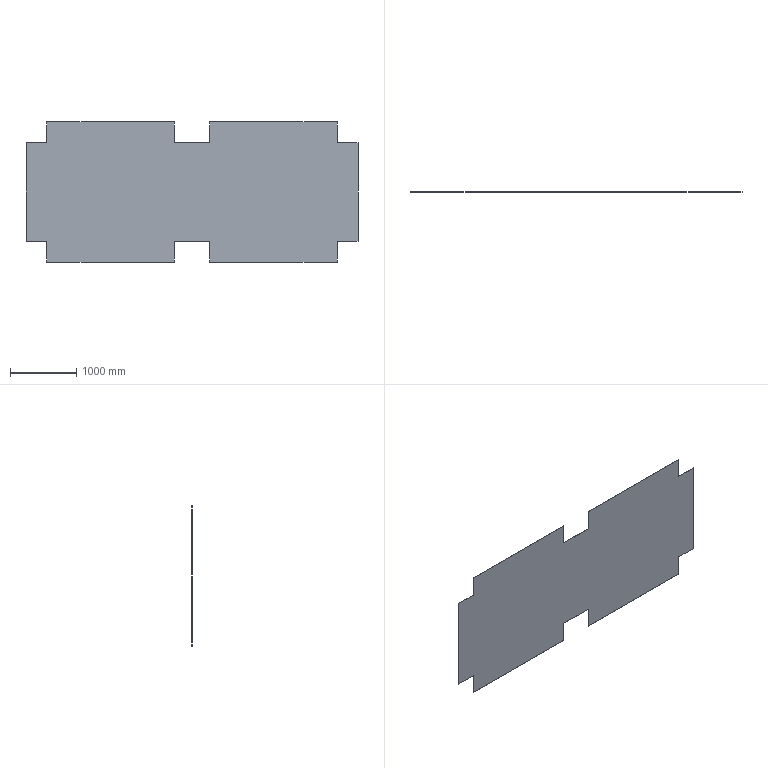Part | SolidWorks | features Extrusion 1 | 1 solid | 22 faces | box 5020 x 3 x 2120 mm | volume 29734800 mm3 | plane 22
STEP:
#1=CARTESIAN_POINT('',(-265.,0.,-1060.));
#2=VERTEX_POINT('',#1);
#3=CARTESIAN_POINT('',(-2195.,0.,-1060.));
#4=VERTEX_POINT('',#3);
#5=CARTESIAN_POINT('',(-265.,0.,-1060.));
#6=DIRECTION('',(-1.,0.,0.));
#7=VECTOR('',#6,1000.);
#8=LINE('',#5,#7);
#9=EDGE_CURVE('',#2,#4,#8,.T.);
#10=ORIENTED_EDGE('',*,*,#9,.T.);
#11=CARTESIAN_POINT('',(-2195.,3.,-1060.));
#12=VERTEX_POINT('',#11);
#13=CARTESIAN_POINT('',(-2195.,3.,-1060.));
#14=DIRECTION('',(0.,-1.,0.));
#15=VECTOR('',#14,1000.);
#16=LINE('',#13,#15);
#17=EDGE_CURVE('',#12,#4,#16,.T.);
#18=ORIENTED_EDGE('',*,*,#17,.F.);
#19=CARTESIAN_POINT('',(-265.,3.,-1060.));
#20=VERTEX_POINT('',#19);
#21=CARTESIAN_POINT('',(-265.,3.,-1060.));
#22=DIRECTION('',(-1.,0.,0.));
#23=VECTOR('',#22,1000.);
#24=LINE('',#21,#23);
#25=EDGE_CURVE('',#20,#12,#24,.T.);
#26=ORIENTED_EDGE('',*,*,#25,.F.);
#27=CARTESIAN_POINT('',(-265.,3.,-1060.));
#28=DIRECTION('',(0.,-1.,0.));
#29=VECTOR('',#28,1000.);
#30=LINE('',#27,#29);
#31=EDGE_CURVE('',#20,#2,#30,.T.);
#32=ORIENTED_EDGE('',*,*,#31,.T.);
#33=EDGE_LOOP('',(#10,#18,#26,#32));
#34=FACE_OUTER_BOUND('',#33,.T.);
#35=CARTESIAN_POINT('',(-265.,3.,-1060.));
#36=DIRECTION('',(0.,0.,1.));
#37=DIRECTION('',(1.,0.,0.));
#38=AXIS2_PLACEMENT_3D('',#35,#36,#37);
#39=PLANE('',#38);
#40=ADVANCED_FACE('',(#34),#39,.F.);
#41=CARTESIAN_POINT('',(-2195.,0.,-745.));
#42=VERTEX_POINT('',#41);
#43=CARTESIAN_POINT('',(-2195.,0.,-1060.));
#44=DIRECTION('',(0.,0.,1.));
#45=VECTOR('',#44,1000.);
#46=LINE('',#43,#45);
#47=EDGE_CURVE('',#4,#42,#46,.T.);
#48=ORIENTED_EDGE('',*,*,#47,.T.);
#49=CARTESIAN_POINT('',(-2195.,3.,-745.));
#50=VERTEX_POINT('',#49);
#51=CARTESIAN_POINT('',(-2195.,3.,-745.));
#52=DIRECTION('',(0.,-1.,0.));
#53=VECTOR('',#52,1000.);
#54=LINE('',#51,#53);
#55=EDGE_CURVE('',#50,#42,#54,.T.);
#56=ORIENTED_EDGE('',*,*,#55,.F.);
#57=CARTESIAN_POINT('',(-2195.,3.,-1060.));
#58=DIRECTION('',(0.,0.,1.));
#59=VECTOR('',#58,1000.);
#60=LINE('',#57,#59);
#61=EDGE_CURVE('',#12,#50,#60,.T.);
#62=ORIENTED_EDGE('',*,*,#61,.F.);
#63=ORIENTED_EDGE('',*,*,#17,.T.);
#64=EDGE_LOOP('',(#48,#56,#62,#63));
#65=FACE_OUTER_BOUND('',#64,.T.);
#66=CARTESIAN_POINT('',(-2195.,3.,-1060.));
#67=DIRECTION('',(1.,0.,0.));
#68=DIRECTION('',(0.,0.,-1.));
#69=AXIS2_PLACEMENT_3D('',#66,#67,#68);
#70=PLANE('',#69);
#71=ADVANCED_FACE('',(#65),#70,.F.);
#72=CARTESIAN_POINT('',(-2510.,0.,-745.));
#73=VERTEX_POINT('',#72);
#74=CARTESIAN_POINT('',(-2195.,0.,-745.));
#75=DIRECTION('',(-1.,0.,0.));
#76=VECTOR('',#75,1000.);
#77=LINE('',#74,#76);
#78=EDGE_CURVE('',#42,#73,#77,.T.);
#79=ORIENTED_EDGE('',*,*,#78,.T.);
#80=CARTESIAN_POINT('',(-2510.,3.,-745.));
#81=VERTEX_POINT('',#80);
#82=CARTESIAN_POINT('',(-2510.,3.,-745.));
#83=DIRECTION('',(0.,-1.,0.));
#84=VECTOR('',#83,1000.);
#85=LINE('',#82,#84);
#86=EDGE_CURVE('',#81,#73,#85,.T.);
#87=ORIENTED_EDGE('',*,*,#86,.F.);
#88=CARTESIAN_POINT('',(-2195.,3.,-745.));
#89=DIRECTION('',(-1.,0.,0.));
#90=VECTOR('',#89,1000.);
#91=LINE('',#88,#90);
#92=EDGE_CURVE('',#50,#81,#91,.T.);
#93=ORIENTED_EDGE('',*,*,#92,.F.);
#94=ORIENTED_EDGE('',*,*,#55,.T.);
#95=EDGE_LOOP('',(#79,#87,#93,#94));
#96=FACE_OUTER_BOUND('',#95,.T.);
#97=CARTESIAN_POINT('',(-2195.,3.,-745.));
#98=DIRECTION('',(0.,0.,1.));
#99=DIRECTION('',(1.,0.,0.));
#100=AXIS2_PLACEMENT_3D('',#97,#98,#99);
#101=PLANE('',#100);
#102=ADVANCED_FACE('',(#96),#101,.F.);
#103=CARTESIAN_POINT('',(-2510.,0.,745.));
#104=VERTEX_POINT('',#103);
#105=CARTESIAN_POINT('',(-2510.,0.,-745.));
#106=DIRECTION('',(0.,0.,1.));
#107=VECTOR('',#106,1000.);
#108=LINE('',#105,#107);
#109=EDGE_CURVE('',#73,#104,#108,.T.);
#110=ORIENTED_EDGE('',*,*,#109,.T.);
#111=CARTESIAN_POINT('',(-2510.,3.,745.));
#112=VERTEX_POINT('',#111);
#113=CARTESIAN_POINT('',(-2510.,3.,745.));
#114=DIRECTION('',(0.,-1.,0.));
#115=VECTOR('',#114,1000.);
#116=LINE('',#113,#115);
#117=EDGE_CURVE('',#112,#104,#116,.T.);
#118=ORIENTED_EDGE('',*,*,#117,.F.);
#119=CARTESIAN_POINT('',(-2510.,3.,-745.));
#120=DIRECTION('',(0.,0.,1.));
#121=VECTOR('',#120,1000.);
#122=LINE('',#119,#121);
#123=EDGE_CURVE('',#81,#112,#122,.T.);
#124=ORIENTED_EDGE('',*,*,#123,.F.);
#125=ORIENTED_EDGE('',*,*,#86,.T.);
#126=EDGE_LOOP('',(#110,#118,#124,#125));
#127=FACE_OUTER_BOUND('',#126,.T.);
#128=CARTESIAN_POINT('',(-2510.,3.,-745.));
#129=DIRECTION('',(1.,0.,0.));
#130=DIRECTION('',(0.,0.,-1.));
#131=AXIS2_PLACEMENT_3D('',#128,#129,#130);
#132=PLANE('',#131);
#133=ADVANCED_FACE('',(#127),#132,.F.);
#134=CARTESIAN_POINT('',(-2195.,0.,745.));
#135=VERTEX_POINT('',#134);
#136=CARTESIAN_POINT('',(-2195.,0.,745.));
#137=DIRECTION('',(1.,0.,0.));
#138=VECTOR('',#137,1000.);
#139=LINE('',#136,#138);
#140=EDGE_CURVE('',#104,#135,#139,.T.);
#141=ORIENTED_EDGE('',*,*,#140,.T.);
#142=CARTESIAN_POINT('',(-2195.,3.,745.));
#143=VERTEX_POINT('',#142);
#144=CARTESIAN_POINT('',(-2195.,3.,745.));
#145=DIRECTION('',(0.,-1.,0.));
#146=VECTOR('',#145,1000.);
#147=LINE('',#144,#146);
#148=EDGE_CURVE('',#143,#135,#147,.T.);
#149=ORIENTED_EDGE('',*,*,#148,.F.);
#150=CARTESIAN_POINT('',(-2195.,3.,745.));
#151=DIRECTION('',(1.,0.,0.));
#152=VECTOR('',#151,1000.);
#153=LINE('',#150,#152);
#154=EDGE_CURVE('',#112,#143,#153,.T.);
#155=ORIENTED_EDGE('',*,*,#154,.F.);
#156=ORIENTED_EDGE('',*,*,#117,.T.);
#157=EDGE_LOOP('',(#141,#149,#155,#156));
#158=FACE_OUTER_BOUND('',#157,.T.);
#159=CARTESIAN_POINT('',(-2195.,3.,745.));
#160=DIRECTION('',(0.,0.,-1.));
#161=DIRECTION('',(-1.,0.,0.));
#162=AXIS2_PLACEMENT_3D('',#159,#160,#161);
#163=PLANE('',#162);
#164=ADVANCED_FACE('',(#158),#163,.F.);
#165=CARTESIAN_POINT('',(-2195.,0.,1060.));
#166=VERTEX_POINT('',#165);
#167=CARTESIAN_POINT('',(-2195.,0.,1060.));
#168=DIRECTION('',(0.,0.,1.));
#169=VECTOR('',#168,1000.);
#170=LINE('',#167,#169);
#171=EDGE_CURVE('',#135,#166,#170,.T.);
#172=ORIENTED_EDGE('',*,*,#171,.T.);
#173=CARTESIAN_POINT('',(-2195.,3.,1060.));
#174=VERTEX_POINT('',#173);
#175=CARTESIAN_POINT('',(-2195.,3.,1060.));
#176=DIRECTION('',(0.,-1.,0.));
#177=VECTOR('',#176,1000.);
#178=LINE('',#175,#177);
#179=EDGE_CURVE('',#174,#166,#178,.T.);
#180=ORIENTED_EDGE('',*,*,#179,.F.);
#181=CARTESIAN_POINT('',(-2195.,3.,1060.));
#182=DIRECTION('',(0.,0.,1.));
#183=VECTOR('',#182,1000.);
#184=LINE('',#181,#183);
#185=EDGE_CURVE('',#143,#174,#184,.T.);
#186=ORIENTED_EDGE('',*,*,#185,.F.);
#187=ORIENTED_EDGE('',*,*,#148,.T.);
#188=EDGE_LOOP('',(#172,#180,#186,#187));
#189=FACE_OUTER_BOUND('',#188,.T.);
#190=CARTESIAN_POINT('',(-2195.,3.,1060.));
#191=DIRECTION('',(1.,0.,0.));
#192=DIRECTION('',(0.,0.,-1.));
#193=AXIS2_PLACEMENT_3D('',#190,#191,#192);
#194=PLANE('',#193);
#195=ADVANCED_FACE('',(#189),#194,.F.);
#196=CARTESIAN_POINT('',(-265.,0.,1060.));
#197=VERTEX_POINT('',#196);
#198=CARTESIAN_POINT('',(-265.,0.,1060.));
#199=DIRECTION('',(1.,0.,0.));
#200=VECTOR('',#199,1000.);
#201=LINE('',#198,#200);
#202=EDGE_CURVE('',#166,#197,#201,.T.);
#203=ORIENTED_EDGE('',*,*,#202,.T.);
#204=CARTESIAN_POINT('',(-265.,3.,1060.));
#205=VERTEX_POINT('',#204);
#206=CARTESIAN_POINT('',(-265.,3.,1060.));
#207=DIRECTION('',(0.,-1.,0.));
#208=VECTOR('',#207,1000.);
#209=LINE('',#206,#208);
#210=EDGE_CURVE('',#205,#197,#209,.T.);
#211=ORIENTED_EDGE('',*,*,#210,.F.);
#212=CARTESIAN_POINT('',(-265.,3.,1060.));
#213=DIRECTION('',(1.,0.,0.));
#214=VECTOR('',#213,1000.);
#215=LINE('',#212,#214);
#216=EDGE_CURVE('',#174,#205,#215,.T.);
#217=ORIENTED_EDGE('',*,*,#216,.F.);
#218=ORIENTED_EDGE('',*,*,#179,.T.);
#219=EDGE_LOOP('',(#203,#211,#217,#218));
#220=FACE_OUTER_BOUND('',#219,.T.);
#221=CARTESIAN_POINT('',(-265.,3.,1060.));
#222=DIRECTION('',(0.,0.,-1.));
#223=DIRECTION('',(-1.,0.,0.));
#224=AXIS2_PLACEMENT_3D('',#221,#222,#223);
#225=PLANE('',#224);
#226=ADVANCED_FACE('',(#220),#225,.F.);
#227=CARTESIAN_POINT('',(-265.,0.,745.));
#228=VERTEX_POINT('',#227);
#229=CARTESIAN_POINT('',(-265.,0.,1060.));
#230=DIRECTION('',(0.,0.,-1.));
#231=VECTOR('',#230,1000.);
#232=LINE('',#229,#231);
#233=EDGE_CURVE('',#197,#228,#232,.T.);
#234=ORIENTED_EDGE('',*,*,#233,.T.);
#235=CARTESIAN_POINT('',(-265.,3.,745.));
#236=VERTEX_POINT('',#235);
#237=CARTESIAN_POINT('',(-265.,3.,745.));
#238=DIRECTION('',(0.,-1.,0.));
#239=VECTOR('',#238,1000.);
#240=LINE('',#237,#239);
#241=EDGE_CURVE('',#236,#228,#240,.T.);
#242=ORIENTED_EDGE('',*,*,#241,.F.);
#243=CARTESIAN_POINT('',(-265.,3.,1060.));
#244=DIRECTION('',(0.,0.,-1.));
#245=VECTOR('',#244,1000.);
#246=LINE('',#243,#245);
#247=EDGE_CURVE('',#205,#236,#246,.T.);
#248=ORIENTED_EDGE('',*,*,#247,.F.);
#249=ORIENTED_EDGE('',*,*,#210,.T.);
#250=EDGE_LOOP('',(#234,#242,#248,#249));
#251=FACE_OUTER_BOUND('',#250,.T.);
#252=CARTESIAN_POINT('',(-265.,3.,1060.));
#253=DIRECTION('',(-1.,0.,0.));
#254=DIRECTION('',(0.,0.,1.));
#255=AXIS2_PLACEMENT_3D('',#252,#253,#254);
#256=PLANE('',#255);
#257=ADVANCED_FACE('',(#251),#256,.F.);
#258=CARTESIAN_POINT('',(265.,0.,745.));
#259=VERTEX_POINT('',#258);
#260=CARTESIAN_POINT('',(-265.,0.,745.));
#261=DIRECTION('',(1.,0.,0.));
#262=VECTOR('',#261,1000.);
#263=LINE('',#260,#262);
#264=EDGE_CURVE('',#228,#259,#263,.T.);
#265=ORIENTED_EDGE('',*,*,#264,.T.);
#266=CARTESIAN_POINT('',(265.,3.,745.));
#267=VERTEX_POINT('',#266);
#268=CARTESIAN_POINT('',(265.,3.,745.));
#269=DIRECTION('',(0.,-1.,0.));
#270=VECTOR('',#269,1000.);
#271=LINE('',#268,#270);
#272=EDGE_CURVE('',#267,#259,#271,.T.);
#273=ORIENTED_EDGE('',*,*,#272,.F.);
#274=CARTESIAN_POINT('',(-265.,3.,745.));
#275=DIRECTION('',(1.,0.,0.));
#276=VECTOR('',#275,1000.);
#277=LINE('',#274,#276);
#278=EDGE_CURVE('',#236,#267,#277,.T.);
#279=ORIENTED_EDGE('',*,*,#278,.F.);
#280=ORIENTED_EDGE('',*,*,#241,.T.);
#281=EDGE_LOOP('',(#265,#273,#279,#280));
#282=FACE_OUTER_BOUND('',#281,.T.);
#283=CARTESIAN_POINT('',(-265.,3.,745.));
#284=DIRECTION('',(0.,0.,-1.));
#285=DIRECTION('',(-1.,0.,0.));
#286=AXIS2_PLACEMENT_3D('',#283,#284,#285);
#287=PLANE('',#286);
#288=ADVANCED_FACE('',(#282),#287,.F.);
#289=CARTESIAN_POINT('',(265.,0.,1060.));
#290=VERTEX_POINT('',#289);
#291=CARTESIAN_POINT('',(265.,0.,1060.));
#292=DIRECTION('',(0.,0.,1.));
#293=VECTOR('',#292,1000.);
#294=LINE('',#291,#293);
#295=EDGE_CURVE('',#259,#290,#294,.T.);
#296=ORIENTED_EDGE('',*,*,#295,.T.);
#297=CARTESIAN_POINT('',(265.,3.,1060.));
#298=VERTEX_POINT('',#297);
#299=CARTESIAN_POINT('',(265.,3.,1060.));
#300=DIRECTION('',(0.,-1.,0.));
#301=VECTOR('',#300,1000.);
#302=LINE('',#299,#301);
#303=EDGE_CURVE('',#298,#290,#302,.T.);
#304=ORIENTED_EDGE('',*,*,#303,.F.);
#305=CARTESIAN_POINT('',(265.,3.,1060.));
#306=DIRECTION('',(0.,0.,1.));
#307=VECTOR('',#306,1000.);
#308=LINE('',#305,#307);
#309=EDGE_CURVE('',#267,#298,#308,.T.);
#310=ORIENTED_EDGE('',*,*,#309,.F.);
#311=ORIENTED_EDGE('',*,*,#272,.T.);
#312=EDGE_LOOP('',(#296,#304,#310,#311));
#313=FACE_OUTER_BOUND('',#312,.T.);
#314=CARTESIAN_POINT('',(265.,3.,1060.));
#315=DIRECTION('',(1.,0.,0.));
#316=DIRECTION('',(0.,0.,-1.));
#317=AXIS2_PLACEMENT_3D('',#314,#315,#316);
#318=PLANE('',#317);
#319=ADVANCED_FACE('',(#313),#318,.F.);
#320=CARTESIAN_POINT('',(2195.,0.,1060.));
#321=VERTEX_POINT('',#320);
#322=CARTESIAN_POINT('',(2195.,0.,1060.));
#323=DIRECTION('',(1.,0.,0.));
#324=VECTOR('',#323,1000.);
#325=LINE('',#322,#324);
#326=EDGE_CURVE('',#290,#321,#325,.T.);
#327=ORIENTED_EDGE('',*,*,#326,.T.);
#328=CARTESIAN_POINT('',(2195.,3.,1060.));
#329=VERTEX_POINT('',#328);
#330=CARTESIAN_POINT('',(2195.,3.,1060.));
#331=DIRECTION('',(0.,-1.,0.));
#332=VECTOR('',#331,1000.);
#333=LINE('',#330,#332);
#334=EDGE_CURVE('',#329,#321,#333,.T.);
#335=ORIENTED_EDGE('',*,*,#334,.F.);
#336=CARTESIAN_POINT('',(2195.,3.,1060.));
#337=DIRECTION('',(1.,0.,0.));
#338=VECTOR('',#337,1000.);
#339=LINE('',#336,#338);
#340=EDGE_CURVE('',#298,#329,#339,.T.);
#341=ORIENTED_EDGE('',*,*,#340,.F.);
#342=ORIENTED_EDGE('',*,*,#303,.T.);
#343=EDGE_LOOP('',(#327,#335,#341,#342));
#344=FACE_OUTER_BOUND('',#343,.T.);
#345=CARTESIAN_POINT('',(2195.,3.,1060.));
#346=DIRECTION('',(0.,0.,-1.));
#347=DIRECTION('',(-1.,0.,0.));
#348=AXIS2_PLACEMENT_3D('',#345,#346,#347);
#349=PLANE('',#348);
#350=ADVANCED_FACE('',(#344),#349,.F.);
#351=CARTESIAN_POINT('',(2195.,0.,745.));
#352=VERTEX_POINT('',#351);
#353=CARTESIAN_POINT('',(2195.,0.,1060.));
#354=DIRECTION('',(0.,0.,-1.));
#355=VECTOR('',#354,1000.);
#356=LINE('',#353,#355);
#357=EDGE_CURVE('',#321,#352,#356,.T.);
#358=ORIENTED_EDGE('',*,*,#357,.T.);
#359=CARTESIAN_POINT('',(2195.,3.,745.));
#360=VERTEX_POINT('',#359);
#361=CARTESIAN_POINT('',(2195.,3.,745.));
#362=DIRECTION('',(0.,-1.,0.));
#363=VECTOR('',#362,1000.);
#364=LINE('',#361,#363);
#365=EDGE_CURVE('',#360,#352,#364,.T.);
#366=ORIENTED_EDGE('',*,*,#365,.F.);
#367=CARTESIAN_POINT('',(2195.,3.,1060.));
#368=DIRECTION('',(0.,0.,-1.));
#369=VECTOR('',#368,1000.);
#370=LINE('',#367,#369);
#371=EDGE_CURVE('',#329,#360,#370,.T.);
#372=ORIENTED_EDGE('',*,*,#371,.F.);
#373=ORIENTED_EDGE('',*,*,#334,.T.);
#374=EDGE_LOOP('',(#358,#366,#372,#373));
#375=FACE_OUTER_BOUND('',#374,.T.);
#376=CARTESIAN_POINT('',(2195.,3.,1060.));
#377=DIRECTION('',(-1.,0.,0.));
#378=DIRECTION('',(0.,0.,1.));
#379=AXIS2_PLACEMENT_3D('',#376,#377,#378);
#380=PLANE('',#379);
#381=ADVANCED_FACE('',(#375),#380,.F.);
#382=CARTESIAN_POINT('',(2510.,0.,745.));
#383=VERTEX_POINT('',#382);
#384=CARTESIAN_POINT('',(2195.,0.,745.));
#385=DIRECTION('',(1.,0.,0.));
#386=VECTOR('',#385,1000.);
#387=LINE('',#384,#386);
#388=EDGE_CURVE('',#352,#383,#387,.T.);
#389=ORIENTED_EDGE('',*,*,#388,.T.);
#390=CARTESIAN_POINT('',(2510.,3.,745.));
#391=VERTEX_POINT('',#390);
#392=CARTESIAN_POINT('',(2510.,3.,745.));
#393=DIRECTION('',(0.,-1.,0.));
#394=VECTOR('',#393,1000.);
#395=LINE('',#392,#394);
#396=EDGE_CURVE('',#391,#383,#395,.T.);
#397=ORIENTED_EDGE('',*,*,#396,.F.);
#398=CARTESIAN_POINT('',(2195.,3.,745.));
#399=DIRECTION('',(1.,0.,0.));
#400=VECTOR('',#399,1000.);
#401=LINE('',#398,#400);
#402=EDGE_CURVE('',#360,#391,#401,.T.);
#403=ORIENTED_EDGE('',*,*,#402,.F.);
#404=ORIENTED_EDGE('',*,*,#365,.T.);
#405=EDGE_LOOP('',(#389,#397,#403,#404));
#406=FACE_OUTER_BOUND('',#405,.T.);
#407=CARTESIAN_POINT('',(2195.,3.,745.));
#408=DIRECTION('',(0.,0.,-1.));
#409=DIRECTION('',(-1.,0.,0.));
#410=AXIS2_PLACEMENT_3D('',#407,#408,#409);
#411=PLANE('',#410);
#412=ADVANCED_FACE('',(#406),#411,.F.);
#413=CARTESIAN_POINT('',(2510.,0.,-745.));
#414=VERTEX_POINT('',#413);
#415=CARTESIAN_POINT('',(2510.,0.,-745.));
#416=DIRECTION('',(0.,0.,-1.));
#417=VECTOR('',#416,1000.);
#418=LINE('',#415,#417);
#419=EDGE_CURVE('',#383,#414,#418,.T.);
#420=ORIENTED_EDGE('',*,*,#419,.T.);
#421=CARTESIAN_POINT('',(2510.,3.,-745.));
#422=VERTEX_POINT('',#421);
#423=CARTESIAN_POINT('',(2510.,3.,-745.));
#424=DIRECTION('',(0.,-1.,0.));
#425=VECTOR('',#424,1000.);
#426=LINE('',#423,#425);
#427=EDGE_CURVE('',#422,#414,#426,.T.);
#428=ORIENTED_EDGE('',*,*,#427,.F.);
#429=CARTESIAN_POINT('',(2510.,3.,-745.));
#430=DIRECTION('',(0.,0.,-1.));
#431=VECTOR('',#430,1000.);
#432=LINE('',#429,#431);
#433=EDGE_CURVE('',#391,#422,#432,.T.);
#434=ORIENTED_EDGE('',*,*,#433,.F.);
#435=ORIENTED_EDGE('',*,*,#396,.T.);
#436=EDGE_LOOP('',(#420,#428,#434,#435));
#437=FACE_OUTER_BOUND('',#436,.T.);
#438=CARTESIAN_POINT('',(2510.,3.,-745.));
#439=DIRECTION('',(-1.,0.,0.));
#440=DIRECTION('',(0.,0.,1.));
#441=AXIS2_PLACEMENT_3D('',#438,#439,#440);
#442=PLANE('',#441);
#443=ADVANCED_FACE('',(#437),#442,.F.);
#444=CARTESIAN_POINT('',(2195.,0.,-745.));
#445=VERTEX_POINT('',#444);
#446=CARTESIAN_POINT('',(2195.,0.,-745.));
#447=DIRECTION('',(-1.,0.,0.));
#448=VECTOR('',#447,1000.);
#449=LINE('',#446,#448);
#450=EDGE_CURVE('',#414,#445,#449,.T.);
#451=ORIENTED_EDGE('',*,*,#450,.T.);
#452=CARTESIAN_POINT('',(2195.,3.,-745.));
#453=VERTEX_POINT('',#452);
#454=CARTESIAN_POINT('',(2195.,3.,-745.));
#455=DIRECTION('',(0.,-1.,0.));
#456=VECTOR('',#455,1000.);
#457=LINE('',#454,#456);
#458=EDGE_CURVE('',#453,#445,#457,.T.);
#459=ORIENTED_EDGE('',*,*,#458,.F.);
#460=CARTESIAN_POINT('',(2195.,3.,-745.));
#461=DIRECTION('',(-1.,0.,0.));
#462=VECTOR('',#461,1000.);
#463=LINE('',#460,#462);
#464=EDGE_CURVE('',#422,#453,#463,.T.);
#465=ORIENTED_EDGE('',*,*,#464,.F.);
#466=ORIENTED_EDGE('',*,*,#427,.T.);
#467=EDGE_LOOP('',(#451,#459,#465,#466));
#468=FACE_OUTER_BOUND('',#467,.T.);
#469=CARTESIAN_POINT('',(2195.,3.,-745.));
#470=DIRECTION('',(0.,0.,1.));
#471=DIRECTION('',(1.,0.,0.));
#472=AXIS2_PLACEMENT_3D('',#469,#470,#471);
#473=PLANE('',#472);
#474=ADVANCED_FACE('',(#468),#473,.F.);
#475=CARTESIAN_POINT('',(2195.,0.,-1060.));
#476=VERTEX_POINT('',#475);
#477=CARTESIAN_POINT('',(2195.,0.,-1060.));
#478=DIRECTION('',(0.,0.,-1.));
#479=VECTOR('',#478,1000.);
#480=LINE('',#477,#479);
#481=EDGE_CURVE('',#445,#476,#480,.T.);
#482=ORIENTED_EDGE('',*,*,#481,.T.);
#483=CARTESIAN_POINT('',(2195.,3.,-1060.));
#484=VERTEX_POINT('',#483);
#485=CARTESIAN_POINT('',(2195.,3.,-1060.));
#486=DIRECTION('',(0.,-1.,0.));
#487=VECTOR('',#486,1000.);
#488=LINE('',#485,#487);
#489=EDGE_CURVE('',#484,#476,#488,.T.);
#490=ORIENTED_EDGE('',*,*,#489,.F.);
#491=CARTESIAN_POINT('',(2195.,3.,-1060.));
#492=DIRECTION('',(0.,0.,-1.));
#493=VECTOR('',#492,1000.);
#494=LINE('',#491,#493);
#495=EDGE_CURVE('',#453,#484,#494,.T.);
#496=ORIENTED_EDGE('',*,*,#495,.F.);
#497=ORIENTED_EDGE('',*,*,#458,.T.);
#498=EDGE_LOOP('',(#482,#490,#496,#497));
#499=FACE_OUTER_BOUND('',#498,.T.);
#500=CARTESIAN_POINT('',(2195.,3.,-1060.));
#501=DIRECTION('',(-1.,0.,0.));
#502=DIRECTION('',(0.,0.,1.));
#503=AXIS2_PLACEMENT_3D('',#500,#501,#502);
#504=PLANE('',#503);
#505=ADVANCED_FACE('',(#499),#504,.F.);
#506=CARTESIAN_POINT('',(265.,0.,-1060.));
#507=VERTEX_POINT('',#506);
#508=CARTESIAN_POINT('',(2195.,0.,-1060.));
#509=DIRECTION('',(-1.,0.,0.));
#510=VECTOR('',#509,1000.);
#511=LINE('',#508,#510);
#512=EDGE_CURVE('',#476,#507,#511,.T.);
#513=ORIENTED_EDGE('',*,*,#512,.T.);
#514=CARTESIAN_POINT('',(265.,3.,-1060.));
#515=VERTEX_POINT('',#514);
#516=CARTESIAN_POINT('',(265.,3.,-1060.));
#517=DIRECTION('',(0.,-1.,0.));
#518=VECTOR('',#517,1000.);
#519=LINE('',#516,#518);
#520=EDGE_CURVE('',#515,#507,#519,.T.);
#521=ORIENTED_EDGE('',*,*,#520,.F.);
#522=CARTESIAN_POINT('',(2195.,3.,-1060.));
#523=DIRECTION('',(-1.,0.,0.));
#524=VECTOR('',#523,1000.);
#525=LINE('',#522,#524);
#526=EDGE_CURVE('',#484,#515,#525,.T.);
#527=ORIENTED_EDGE('',*,*,#526,.F.);
#528=ORIENTED_EDGE('',*,*,#489,.T.);
#529=EDGE_LOOP('',(#513,#521,#527,#528));
#530=FACE_OUTER_BOUND('',#529,.T.);
#531=CARTESIAN_POINT('',(2195.,3.,-1060.));
#532=DIRECTION('',(0.,0.,1.));
#533=DIRECTION('',(1.,0.,0.));
#534=AXIS2_PLACEMENT_3D('',#531,#532,#533);
#535=PLANE('',#534);
#536=ADVANCED_FACE('',(#530),#535,.F.);
#537=CARTESIAN_POINT('',(265.,0.,-745.));
#538=VERTEX_POINT('',#537);
#539=CARTESIAN_POINT('',(265.,0.,-1060.));
#540=DIRECTION('',(0.,0.,1.));
#541=VECTOR('',#540,1000.);
#542=LINE('',#539,#541);
#543=EDGE_CURVE('',#507,#538,#542,.T.);
#544=ORIENTED_EDGE('',*,*,#543,.T.);
#545=CARTESIAN_POINT('',(265.,3.,-745.));
#546=VERTEX_POINT('',#545);
#547=CARTESIAN_POINT('',(265.,3.,-745.));
#548=DIRECTION('',(0.,-1.,0.));
#549=VECTOR('',#548,1000.);
#550=LINE('',#547,#549);
#551=EDGE_CURVE('',#546,#538,#550,.T.);
#552=ORIENTED_EDGE('',*,*,#551,.F.);
#553=CARTESIAN_POINT('',(265.,3.,-1060.));
#554=DIRECTION('',(0.,0.,1.));
#555=VECTOR('',#554,1000.);
#556=LINE('',#553,#555);
#557=EDGE_CURVE('',#515,#546,#556,.T.);
#558=ORIENTED_EDGE('',*,*,#557,.F.);
#559=ORIENTED_EDGE('',*,*,#520,.T.);
#560=EDGE_LOOP('',(#544,#552,#558,#559));
#561=FACE_OUTER_BOUND('',#560,.T.);
#562=CARTESIAN_POINT('',(265.,3.,-1060.));
#563=DIRECTION('',(1.,0.,0.));
#564=DIRECTION('',(0.,0.,-1.));
#565=AXIS2_PLACEMENT_3D('',#562,#563,#564);
#566=PLANE('',#565);
#567=ADVANCED_FACE('',(#561),#566,.F.);
#568=CARTESIAN_POINT('',(-265.,0.,-745.));
#569=VERTEX_POINT('',#568);
#570=CARTESIAN_POINT('',(-265.,0.,-745.));
#571=DIRECTION('',(-1.,0.,0.));
#572=VECTOR('',#571,1000.);
#573=LINE('',#570,#572);
#574=EDGE_CURVE('',#538,#569,#573,.T.);
#575=ORIENTED_EDGE('',*,*,#574,.T.);
#576=CARTESIAN_POINT('',(-265.,3.,-745.));
#577=VERTEX_POINT('',#576);
#578=CARTESIAN_POINT('',(-265.,3.,-745.));
#579=DIRECTION('',(0.,-1.,0.));
#580=VECTOR('',#579,1000.);
#581=LINE('',#578,#580);
#582=EDGE_CURVE('',#577,#569,#581,.T.);
#583=ORIENTED_EDGE('',*,*,#582,.F.);
#584=CARTESIAN_POINT('',(-265.,3.,-745.));
#585=DIRECTION('',(-1.,0.,0.));
#586=VECTOR('',#585,1000.);
#587=LINE('',#584,#586);
#588=EDGE_CURVE('',#546,#577,#587,.T.);
#589=ORIENTED_EDGE('',*,*,#588,.F.);
#590=ORIENTED_EDGE('',*,*,#551,.T.);
#591=EDGE_LOOP('',(#575,#583,#589,#590));
#592=FACE_OUTER_BOUND('',#591,.T.);
#593=CARTESIAN_POINT('',(-265.,3.,-745.));
#594=DIRECTION('',(0.,0.,1.));
#595=DIRECTION('',(1.,0.,0.));
#596=AXIS2_PLACEMENT_3D('',#593,#594,#595);
#597=PLANE('',#596);
#598=ADVANCED_FACE('',(#592),#597,.F.);
#599=CARTESIAN_POINT('',(-265.,0.,-1060.));
#600=DIRECTION('',(0.,0.,-1.));
#601=VECTOR('',#600,1000.);
#602=LINE('',#599,#601);
#603=EDGE_CURVE('',#569,#2,#602,.T.);
#604=ORIENTED_EDGE('',*,*,#603,.T.);
#605=ORIENTED_EDGE('',*,*,#31,.F.);
#606=CARTESIAN_POINT('',(-265.,3.,-1060.));
#607=DIRECTION('',(0.,0.,-1.));
#608=VECTOR('',#607,1000.);
#609=LINE('',#606,#608);
#610=EDGE_CURVE('',#577,#20,#609,.T.);
#611=ORIENTED_EDGE('',*,*,#610,.F.);
#612=ORIENTED_EDGE('',*,*,#582,.T.);
#613=EDGE_LOOP('',(#604,#605,#611,#612));
#614=FACE_OUTER_BOUND('',#613,.T.);
#615=CARTESIAN_POINT('',(-265.,3.,-1060.));
#616=DIRECTION('',(-1.,0.,0.));
#617=DIRECTION('',(0.,0.,1.));
#618=AXIS2_PLACEMENT_3D('',#615,#616,#617);
#619=PLANE('',#618);
#620=ADVANCED_FACE('',(#614),#619,.F.);
#621=ORIENTED_EDGE('',*,*,#25,.T.);
#622=ORIENTED_EDGE('',*,*,#61,.T.);
#623=ORIENTED_EDGE('',*,*,#92,.T.);
#624=ORIENTED_EDGE('',*,*,#123,.T.);
#625=ORIENTED_EDGE('',*,*,#154,.T.);
#626=ORIENTED_EDGE('',*,*,#185,.T.);
#627=ORIENTED_EDGE('',*,*,#216,.T.);
#628=ORIENTED_EDGE('',*,*,#247,.T.);
#629=ORIENTED_EDGE('',*,*,#278,.T.);
#630=ORIENTED_EDGE('',*,*,#309,.T.);
#631=ORIENTED_EDGE('',*,*,#340,.T.);
#632=ORIENTED_EDGE('',*,*,#371,.T.);
#633=ORIENTED_EDGE('',*,*,#402,.T.);
#634=ORIENTED_EDGE('',*,*,#433,.T.);
#635=ORIENTED_EDGE('',*,*,#464,.T.);
#636=ORIENTED_EDGE('',*,*,#495,.T.);
#637=ORIENTED_EDGE('',*,*,#526,.T.);
#638=ORIENTED_EDGE('',*,*,#557,.T.);
#639=ORIENTED_EDGE('',*,*,#588,.T.);
#640=ORIENTED_EDGE('',*,*,#610,.T.);
#641=EDGE_LOOP('',(#621,#622,#623,#624,#625,#626,#627,#628,#629,#630,#631,#632,#633,#634,#635,#636,#637,#638,#639,#640));
#642=FACE_OUTER_BOUND('',#641,.T.);
#643=CARTESIAN_POINT('',(0.,3.,0.));
#644=DIRECTION('',(0.,1.,0.));
#645=DIRECTION('',(0.,0.,1.));
#646=AXIS2_PLACEMENT_3D('',#643,#644,#645);
#647=PLANE('',#646);
#648=ADVANCED_FACE('',(#642),#647,.T.);
#649=ORIENTED_EDGE('',*,*,#9,.F.);
#650=ORIENTED_EDGE('',*,*,#603,.F.);
#651=ORIENTED_EDGE('',*,*,#574,.F.);
#652=ORIENTED_EDGE('',*,*,#543,.F.);
#653=ORIENTED_EDGE('',*,*,#512,.F.);
#654=ORIENTED_EDGE('',*,*,#481,.F.);
#655=ORIENTED_EDGE('',*,*,#450,.F.);
#656=ORIENTED_EDGE('',*,*,#419,.F.);
#657=ORIENTED_EDGE('',*,*,#388,.F.);
#658=ORIENTED_EDGE('',*,*,#357,.F.);
#659=ORIENTED_EDGE('',*,*,#326,.F.);
#660=ORIENTED_EDGE('',*,*,#295,.F.);
#661=ORIENTED_EDGE('',*,*,#264,.F.);
#662=ORIENTED_EDGE('',*,*,#233,.F.);
#663=ORIENTED_EDGE('',*,*,#202,.F.);
#664=ORIENTED_EDGE('',*,*,#171,.F.);
#665=ORIENTED_EDGE('',*,*,#140,.F.);
#666=ORIENTED_EDGE('',*,*,#109,.F.);
#667=ORIENTED_EDGE('',*,*,#78,.F.);
#668=ORIENTED_EDGE('',*,*,#47,.F.);
#669=EDGE_LOOP('',(#649,#650,#651,#652,#653,#654,#655,#656,#657,#658,#659,#660,#661,#662,#663,#664,#665,#666,#667,#668));
#670=FACE_OUTER_BOUND('',#669,.T.);
#671=CARTESIAN_POINT('',(0.,0.,0.));
#672=DIRECTION('',(0.,1.,0.));
#673=DIRECTION('',(0.,0.,1.));
#674=AXIS2_PLACEMENT_3D('',#671,#672,#673);
#675=PLANE('',#674);
#676=ADVANCED_FACE('',(#670),#675,.F.);
#677=CLOSED_SHELL('',(#40,#71,#102,#133,#164,#195,#226,#257,#288,#319,#350,#381,#412,#443,#474,#505,#536,#567,#598,#620,#648,#676));
#678=MANIFOLD_SOLID_BREP('',#677);
#679=CARTESIAN_POINT('',(0.,0.,0.));
#680=DIRECTION('',(0.,0.,1.));
#681=DIRECTION('',(1.,0.,0.));
#682=AXIS2_PLACEMENT_3D('',#679,#680,#681);
#683=(LENGTH_UNIT()NAMED_UNIT(*)SI_UNIT(.MILLI.,.METRE.));
#684=UNCERTAINTY_MEASURE_WITH_UNIT(LENGTH_MEASURE(0.00001),#683,'','');
#685=(NAMED_UNIT(*)PLANE_ANGLE_UNIT()SI_UNIT($,.RADIAN.));
#686=(NAMED_UNIT(*)SI_UNIT($,.STERADIAN.)SOLID_ANGLE_UNIT());
#687=(GEOMETRIC_REPRESENTATION_CONTEXT(3)GLOBAL_UNCERTAINTY_ASSIGNED_CONTEXT((#684))GLOBAL_UNIT_ASSIGNED_CONTEXT((#683,#685,#686))REPRESENTATION_CONTEXT('',''));
#688=ADVANCED_BREP_SHAPE_REPRESENTATION('',(#678,#682),#687);